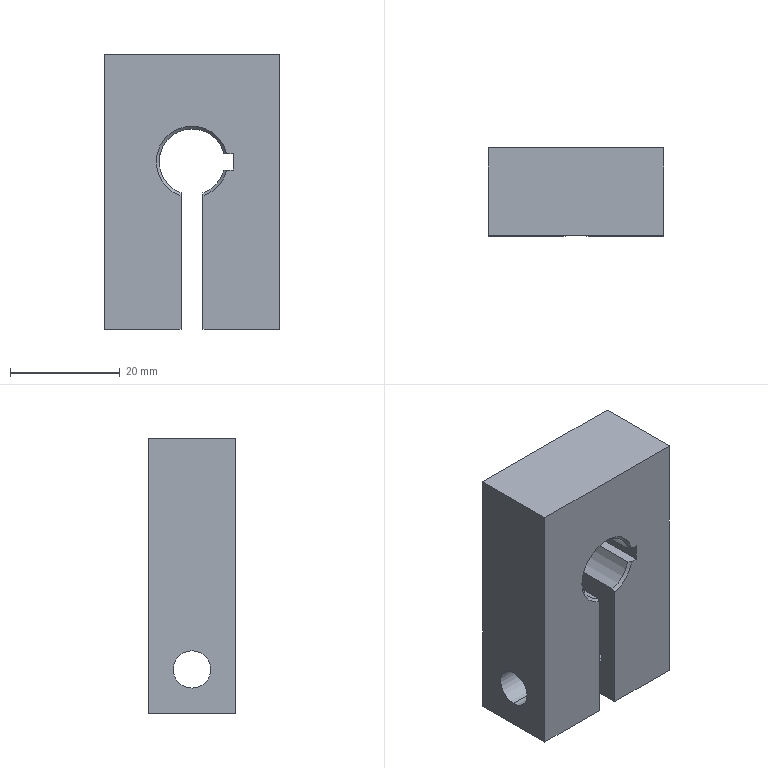Part | SolidWorks | features Chamfer 2, ICE 2, FlatPattern 1, HoleWzd 1, SMBaseFlange 1, SheetMetal 1 | 1 solid | 25 faces | box 32 x 16 x 50 mm | volume 20733 mm3 | plane 14 | cylinder 6 | cone 5 | commonest cylinder face diameters 6.8 x2 9 x2 12 x2
STEP:
#1=CARTESIAN_POINT('',(16.,15.5,-13.5));
#2=VERTEX_POINT('',#1);
#3=CARTESIAN_POINT('',(21.809,15.5,-18.));
#4=VERTEX_POINT('',#3);
#5=CARTESIAN_POINT('',(16.,15.5,-19.5));
#6=DIRECTION('',(0.,1.,0.));
#7=DIRECTION('',(0.,0.,1.));
#8=AXIS2_PLACEMENT_3D('',#5,#6,#7);
#9=CIRCLE('',#8,6.);
#10=EDGE_CURVE('',#2,#4,#9,.T.);
#11=ORIENTED_EDGE('',*,*,#10,.F.);
#12=CARTESIAN_POINT('',(16.,16.,-13.));
#13=VERTEX_POINT('',#12);
#14=CARTESIAN_POINT('',(16.,16.,-13.));
#15=DIRECTION('',(0.,0.7071,0.7071));
#16=VECTOR('',#15,1000.);
#17=LINE('',#14,#16);
#18=EDGE_CURVE('',#2,#13,#17,.T.);
#19=ORIENTED_EDGE('',*,*,#18,.T.);
#20=CARTESIAN_POINT('',(22.246,16.,-17.7));
#21=VERTEX_POINT('',#20);
#22=CARTESIAN_POINT('',(16.,16.,-19.5));
#23=DIRECTION('',(0.,-1.,0.));
#24=DIRECTION('',(0.,0.,1.));
#25=AXIS2_PLACEMENT_3D('',#22,#23,#24);
#26=CIRCLE('',#25,6.5);
#27=EDGE_CURVE('',#21,#13,#26,.T.);
#28=ORIENTED_EDGE('',*,*,#27,.F.);
#29=CARTESIAN_POINT('',(22.016,15.7,-18.));
#30=VERTEX_POINT('',#29);
#31=CARTESIAN_POINT('',(22.246,16.,-17.7));
#32=CARTESIAN_POINT('',(22.17,15.9,-17.8));
#33=CARTESIAN_POINT('',(22.094,15.8,-17.9));
#34=CARTESIAN_POINT('',(22.016,15.7,-18.));
#35=B_SPLINE_CURVE_WITH_KNOTS('',3,(#31,#32,#33,#34),.UNSPECIFIED.,.F.,.F.,(4,4),(0.,0.0004826),.UNSPECIFIED.);
#36=EDGE_CURVE('',#21,#30,#35,.T.);
#37=ORIENTED_EDGE('',*,*,#36,.T.);
#38=CARTESIAN_POINT('',(21.809,15.5,-18.));
#39=CARTESIAN_POINT('',(21.878,15.567,-18.));
#40=CARTESIAN_POINT('',(21.947,15.633,-18.));
#41=CARTESIAN_POINT('',(22.016,15.7,-18.));
#42=B_SPLINE_CURVE_WITH_KNOTS('',3,(#38,#39,#40,#41),.UNSPECIFIED.,.F.,.F.,(4,4),(0.,0.0002874),.UNSPECIFIED.);
#43=EDGE_CURVE('',#4,#30,#42,.T.);
#44=ORIENTED_EDGE('',*,*,#43,.F.);
#45=EDGE_LOOP('',(#11,#19,#28,#37,#44));
#46=FACE_OUTER_BOUND('',#45,.T.);
#47=CARTESIAN_POINT('',(16.,16.,-19.5));
#48=DIRECTION('',(0.,1.,0.));
#49=DIRECTION('',(0.,0.,1.));
#50=AXIS2_PLACEMENT_3D('',#47,#48,#49);
#51=CONICAL_SURFACE('',#50,6.5,0.7854);
#52=ADVANCED_FACE('',(#46),#51,.F.);
#53=CARTESIAN_POINT('',(14.,8.,-45.4));
#54=VERTEX_POINT('',#53);
#55=CARTESIAN_POINT('',(14.,8.,-38.6));
#56=VERTEX_POINT('',#55);
#57=CARTESIAN_POINT('',(14.,8.,-42.));
#58=DIRECTION('',(-1.,0.,0.));
#59=DIRECTION('',(0.,0.,1.));
#60=AXIS2_PLACEMENT_3D('',#57,#58,#59);
#61=CIRCLE('',#60,3.4);
#62=EDGE_CURVE('',#54,#56,#61,.T.);
#63=ORIENTED_EDGE('',*,*,#62,.F.);
#64=CARTESIAN_POINT('',(0.,8.,-45.4));
#65=VERTEX_POINT('',#64);
#66=CARTESIAN_POINT('',(0.,8.,-45.4));
#67=DIRECTION('',(-1.,0.,0.));
#68=VECTOR('',#67,1000.);
#69=LINE('',#66,#68);
#70=EDGE_CURVE('',#54,#65,#69,.T.);
#71=ORIENTED_EDGE('',*,*,#70,.T.);
#72=CARTESIAN_POINT('',(0.,8.,-38.6));
#73=VERTEX_POINT('',#72);
#74=CARTESIAN_POINT('',(0.,8.,-42.));
#75=DIRECTION('',(-1.,0.,0.));
#76=DIRECTION('',(0.,0.,1.));
#77=AXIS2_PLACEMENT_3D('',#74,#75,#76);
#78=CIRCLE('',#77,3.4);
#79=EDGE_CURVE('',#65,#73,#78,.T.);
#80=ORIENTED_EDGE('',*,*,#79,.T.);
#81=CARTESIAN_POINT('',(0.,8.,-38.6));
#82=DIRECTION('',(-1.,0.,0.));
#83=VECTOR('',#82,1000.);
#84=LINE('',#81,#83);
#85=EDGE_CURVE('',#56,#73,#84,.T.);
#86=ORIENTED_EDGE('',*,*,#85,.F.);
#87=EDGE_LOOP('',(#63,#71,#80,#86));
#88=FACE_OUTER_BOUND('',#87,.T.);
#89=CARTESIAN_POINT('',(0.,8.,-42.));
#90=DIRECTION('',(-1.,0.,0.));
#91=DIRECTION('',(0.,0.,1.));
#92=AXIS2_PLACEMENT_3D('',#89,#90,#91);
#93=CYLINDRICAL_SURFACE('',#92,3.4);
#94=ADVANCED_FACE('',(#88),#93,.F.);
#95=CARTESIAN_POINT('',(18.,8.,-46.5));
#96=VERTEX_POINT('',#95);
#97=CARTESIAN_POINT('',(18.,8.,-37.5));
#98=VERTEX_POINT('',#97);
#99=CARTESIAN_POINT('',(18.,8.,-42.));
#100=DIRECTION('',(-1.,0.,0.));
#101=DIRECTION('',(0.,0.,-1.));
#102=AXIS2_PLACEMENT_3D('',#99,#100,#101);
#103=CIRCLE('',#102,4.5);
#104=EDGE_CURVE('',#96,#98,#103,.T.);
#105=ORIENTED_EDGE('',*,*,#104,.T.);
#106=CARTESIAN_POINT('',(32.,8.,-37.5));
#107=VERTEX_POINT('',#106);
#108=CARTESIAN_POINT('',(-0.001,8.,-37.5));
#109=DIRECTION('',(1.,0.,0.));
#110=VECTOR('',#109,1000.);
#111=LINE('',#108,#110);
#112=EDGE_CURVE('',#98,#107,#111,.T.);
#113=ORIENTED_EDGE('',*,*,#112,.T.);
#114=CARTESIAN_POINT('',(32.,8.,-46.5));
#115=VERTEX_POINT('',#114);
#116=CARTESIAN_POINT('',(32.,8.,-42.));
#117=DIRECTION('',(1.,0.,0.));
#118=DIRECTION('',(0.,0.,-1.));
#119=AXIS2_PLACEMENT_3D('',#116,#117,#118);
#120=CIRCLE('',#119,4.5);
#121=EDGE_CURVE('',#107,#115,#120,.T.);
#122=ORIENTED_EDGE('',*,*,#121,.T.);
#123=CARTESIAN_POINT('',(-0.001,8.,-46.5));
#124=DIRECTION('',(1.,0.,0.));
#125=VECTOR('',#124,1000.);
#126=LINE('',#123,#125);
#127=EDGE_CURVE('',#96,#115,#126,.T.);
#128=ORIENTED_EDGE('',*,*,#127,.F.);
#129=EDGE_LOOP('',(#105,#113,#122,#128));
#130=FACE_OUTER_BOUND('',#129,.T.);
#131=CARTESIAN_POINT('',(-0.001,8.,-42.));
#132=DIRECTION('',(1.,0.,0.));
#133=DIRECTION('',(0.,0.,-1.));
#134=AXIS2_PLACEMENT_3D('',#131,#132,#133);
#135=CYLINDRICAL_SURFACE('',#134,4.5);
#136=ADVANCED_FACE('',(#130),#135,.F.);
#137=CARTESIAN_POINT('',(0.,8.,-42.));
#138=DIRECTION('',(-1.,0.,0.));
#139=DIRECTION('',(0.,0.,1.));
#140=AXIS2_PLACEMENT_3D('',#137,#138,#139);
#141=CIRCLE('',#140,3.4);
#142=EDGE_CURVE('',#73,#65,#141,.T.);
#143=ORIENTED_EDGE('',*,*,#142,.F.);
#144=ORIENTED_EDGE('',*,*,#79,.F.);
#145=EDGE_LOOP('',(#143,#144));
#146=FACE_BOUND('',#145,.T.);
#147=CARTESIAN_POINT('',(0.,0.,-50.));
#148=VERTEX_POINT('',#147);
#149=CARTESIAN_POINT('',(0.,0.,0.));
#150=VERTEX_POINT('',#149);
#151=CARTESIAN_POINT('',(0.,0.,0.));
#152=DIRECTION('',(0.,0.,1.));
#153=VECTOR('',#152,1000.);
#154=LINE('',#151,#153);
#155=EDGE_CURVE('',#148,#150,#154,.T.);
#156=ORIENTED_EDGE('',*,*,#155,.T.);
#157=CARTESIAN_POINT('',(0.,16.,0.));
#158=VERTEX_POINT('',#157);
#159=CARTESIAN_POINT('',(0.,16.,0.));
#160=DIRECTION('',(0.,-1.,0.));
#161=VECTOR('',#160,1000.);
#162=LINE('',#159,#161);
#163=EDGE_CURVE('',#158,#150,#162,.T.);
#164=ORIENTED_EDGE('',*,*,#163,.F.);
#165=CARTESIAN_POINT('',(0.,16.,-50.));
#166=VERTEX_POINT('',#165);
#167=CARTESIAN_POINT('',(0.,16.,0.));
#168=DIRECTION('',(0.,0.,1.));
#169=VECTOR('',#168,1000.);
#170=LINE('',#167,#169);
#171=EDGE_CURVE('',#166,#158,#170,.T.);
#172=ORIENTED_EDGE('',*,*,#171,.F.);
#173=CARTESIAN_POINT('',(0.,16.,-50.));
#174=DIRECTION('',(0.,-1.,0.));
#175=VECTOR('',#174,1000.);
#176=LINE('',#173,#175);
#177=EDGE_CURVE('',#166,#148,#176,.T.);
#178=ORIENTED_EDGE('',*,*,#177,.T.);
#179=EDGE_LOOP('',(#156,#164,#172,#178));
#180=FACE_OUTER_BOUND('',#179,.T.);
#181=CARTESIAN_POINT('',(0.,16.,0.));
#182=DIRECTION('',(1.,0.,0.));
#183=DIRECTION('',(0.,0.,-1.));
#184=AXIS2_PLACEMENT_3D('',#181,#182,#183);
#185=PLANE('',#184);
#186=ADVANCED_FACE('',(#146,#180),#185,.F.);
#187=CARTESIAN_POINT('',(32.,0.,0.));
#188=VERTEX_POINT('',#187);
#189=CARTESIAN_POINT('',(0.,0.,0.));
#190=DIRECTION('',(1.,0.,0.));
#191=VECTOR('',#190,1000.);
#192=LINE('',#189,#191);
#193=EDGE_CURVE('',#150,#188,#192,.T.);
#194=ORIENTED_EDGE('',*,*,#193,.T.);
#195=CARTESIAN_POINT('',(32.,16.,0.));
#196=VERTEX_POINT('',#195);
#197=CARTESIAN_POINT('',(32.,16.,0.));
#198=DIRECTION('',(0.,-1.,0.));
#199=VECTOR('',#198,1000.);
#200=LINE('',#197,#199);
#201=EDGE_CURVE('',#196,#188,#200,.T.);
#202=ORIENTED_EDGE('',*,*,#201,.F.);
#203=CARTESIAN_POINT('',(0.,16.,0.));
#204=DIRECTION('',(1.,0.,0.));
#205=VECTOR('',#204,1000.);
#206=LINE('',#203,#205);
#207=EDGE_CURVE('',#158,#196,#206,.T.);
#208=ORIENTED_EDGE('',*,*,#207,.F.);
#209=ORIENTED_EDGE('',*,*,#163,.T.);
#210=EDGE_LOOP('',(#194,#202,#208,#209));
#211=FACE_OUTER_BOUND('',#210,.T.);
#212=CARTESIAN_POINT('',(0.,16.,0.));
#213=DIRECTION('',(0.,0.,-1.));
#214=DIRECTION('',(-1.,0.,0.));
#215=AXIS2_PLACEMENT_3D('',#212,#213,#214);
#216=PLANE('',#215);
#217=ADVANCED_FACE('',(#211),#216,.F.);
#218=CARTESIAN_POINT('',(32.,8.,-42.));
#219=DIRECTION('',(1.,0.,0.));
#220=DIRECTION('',(0.,0.,-1.));
#221=AXIS2_PLACEMENT_3D('',#218,#219,#220);
#222=CIRCLE('',#221,4.5);
#223=EDGE_CURVE('',#115,#107,#222,.T.);
#224=ORIENTED_EDGE('',*,*,#223,.F.);
#225=ORIENTED_EDGE('',*,*,#121,.F.);
#226=EDGE_LOOP('',(#224,#225));
#227=FACE_BOUND('',#226,.T.);
#228=CARTESIAN_POINT('',(32.,0.,-50.));
#229=VERTEX_POINT('',#228);
#230=CARTESIAN_POINT('',(32.,0.,0.));
#231=DIRECTION('',(0.,0.,-1.));
#232=VECTOR('',#231,1000.);
#233=LINE('',#230,#232);
#234=EDGE_CURVE('',#188,#229,#233,.T.);
#235=ORIENTED_EDGE('',*,*,#234,.T.);
#236=CARTESIAN_POINT('',(32.,16.,-50.));
#237=VERTEX_POINT('',#236);
#238=CARTESIAN_POINT('',(32.,16.,-50.));
#239=DIRECTION('',(0.,-1.,0.));
#240=VECTOR('',#239,1000.);
#241=LINE('',#238,#240);
#242=EDGE_CURVE('',#237,#229,#241,.T.);
#243=ORIENTED_EDGE('',*,*,#242,.F.);
#244=CARTESIAN_POINT('',(32.,16.,0.));
#245=DIRECTION('',(0.,0.,-1.));
#246=VECTOR('',#245,1000.);
#247=LINE('',#244,#246);
#248=EDGE_CURVE('',#196,#237,#247,.T.);
#249=ORIENTED_EDGE('',*,*,#248,.F.);
#250=ORIENTED_EDGE('',*,*,#201,.T.);
#251=EDGE_LOOP('',(#235,#243,#249,#250));
#252=FACE_OUTER_BOUND('',#251,.T.);
#253=CARTESIAN_POINT('',(32.,16.,0.));
#254=DIRECTION('',(-1.,0.,0.));
#255=DIRECTION('',(0.,0.,1.));
#256=AXIS2_PLACEMENT_3D('',#253,#254,#255);
#257=PLANE('',#256);
#258=ADVANCED_FACE('',(#227,#252),#257,.F.);
#259=CARTESIAN_POINT('',(18.,0.,-50.));
#260=VERTEX_POINT('',#259);
#261=CARTESIAN_POINT('',(18.,0.,-50.));
#262=DIRECTION('',(-1.,0.,0.));
#263=VECTOR('',#262,1000.);
#264=LINE('',#261,#263);
#265=EDGE_CURVE('',#229,#260,#264,.T.);
#266=ORIENTED_EDGE('',*,*,#265,.T.);
#267=CARTESIAN_POINT('',(18.,16.,-50.));
#268=VERTEX_POINT('',#267);
#269=CARTESIAN_POINT('',(18.,16.,-50.));
#270=DIRECTION('',(0.,-1.,0.));
#271=VECTOR('',#270,1000.);
#272=LINE('',#269,#271);
#273=EDGE_CURVE('',#268,#260,#272,.T.);
#274=ORIENTED_EDGE('',*,*,#273,.F.);
#275=CARTESIAN_POINT('',(18.,16.,-50.));
#276=DIRECTION('',(-1.,0.,0.));
#277=VECTOR('',#276,1000.);
#278=LINE('',#275,#277);
#279=EDGE_CURVE('',#237,#268,#278,.T.);
#280=ORIENTED_EDGE('',*,*,#279,.F.);
#281=ORIENTED_EDGE('',*,*,#242,.T.);
#282=EDGE_LOOP('',(#266,#274,#280,#281));
#283=FACE_OUTER_BOUND('',#282,.T.);
#284=CARTESIAN_POINT('',(18.,16.,-50.));
#285=DIRECTION('',(0.,0.,1.));
#286=DIRECTION('',(1.,0.,0.));
#287=AXIS2_PLACEMENT_3D('',#284,#285,#286);
#288=PLANE('',#287);
#289=ADVANCED_FACE('',(#283),#288,.F.);
#290=ORIENTED_EDGE('',*,*,#104,.F.);
#291=CARTESIAN_POINT('',(18.,8.,-42.));
#292=DIRECTION('',(-1.,0.,0.));
#293=DIRECTION('',(0.,0.,-1.));
#294=AXIS2_PLACEMENT_3D('',#291,#292,#293);
#295=CIRCLE('',#294,4.5);
#296=EDGE_CURVE('',#98,#96,#295,.T.);
#297=ORIENTED_EDGE('',*,*,#296,.F.);
#298=EDGE_LOOP('',(#290,#297));
#299=FACE_BOUND('',#298,.T.);
#300=CARTESIAN_POINT('',(18.,0.,-25.685));
#301=VERTEX_POINT('',#300);
#302=CARTESIAN_POINT('',(18.,0.,-50.));
#303=DIRECTION('',(0.,0.,1.));
#304=VECTOR('',#303,1000.);
#305=LINE('',#302,#304);
#306=EDGE_CURVE('',#260,#301,#305,.T.);
#307=ORIENTED_EDGE('',*,*,#306,.T.);
#308=CARTESIAN_POINT('',(18.,0.5,-25.157));
#309=VERTEX_POINT('',#308);
#310=CARTESIAN_POINT('',(18.,0.,-25.685));
#311=CARTESIAN_POINT('',(18.,0.1671,-25.509));
#312=CARTESIAN_POINT('',(18.,0.3338,-25.333));
#313=CARTESIAN_POINT('',(18.,0.5,-25.157));
#314=B_SPLINE_CURVE_WITH_KNOTS('',3,(#310,#311,#312,#313),.UNSPECIFIED.,.F.,.F.,(4,4),(0.,0.000727),.UNSPECIFIED.);
#315=EDGE_CURVE('',#301,#309,#314,.T.);
#316=ORIENTED_EDGE('',*,*,#315,.T.);
#317=CARTESIAN_POINT('',(18.,15.5,-25.157));
#318=VERTEX_POINT('',#317);
#319=CARTESIAN_POINT('',(18.,16.,-25.157));
#320=DIRECTION('',(0.,-1.,0.));
#321=VECTOR('',#320,1000.);
#322=LINE('',#319,#321);
#323=EDGE_CURVE('',#318,#309,#322,.T.);
#324=ORIENTED_EDGE('',*,*,#323,.F.);
#325=CARTESIAN_POINT('',(18.,16.,-25.685));
#326=VERTEX_POINT('',#325);
#327=CARTESIAN_POINT('',(18.,15.5,-25.157));
#328=CARTESIAN_POINT('',(18.,15.666,-25.333));
#329=CARTESIAN_POINT('',(18.,15.833,-25.509));
#330=CARTESIAN_POINT('',(18.,16.,-25.685));
#331=B_SPLINE_CURVE_WITH_KNOTS('',3,(#327,#328,#329,#330),.UNSPECIFIED.,.F.,.F.,(4,4),(0.,0.000727),.UNSPECIFIED.);
#332=EDGE_CURVE('',#318,#326,#331,.T.);
#333=ORIENTED_EDGE('',*,*,#332,.T.);
#334=CARTESIAN_POINT('',(18.,16.,-50.));
#335=DIRECTION('',(0.,0.,1.));
#336=VECTOR('',#335,1000.);
#337=LINE('',#334,#336);
#338=EDGE_CURVE('',#268,#326,#337,.T.);
#339=ORIENTED_EDGE('',*,*,#338,.F.);
#340=ORIENTED_EDGE('',*,*,#273,.T.);
#341=EDGE_LOOP('',(#307,#316,#324,#333,#339,#340));
#342=FACE_OUTER_BOUND('',#341,.T.);
#343=CARTESIAN_POINT('',(18.,16.,-50.));
#344=DIRECTION('',(1.,0.,0.));
#345=DIRECTION('',(0.,0.,-1.));
#346=AXIS2_PLACEMENT_3D('',#343,#344,#345);
#347=PLANE('',#346);
#348=ADVANCED_FACE('',(#299,#342),#347,.F.);
#349=ORIENTED_EDGE('',*,*,#323,.T.);
#350=CARTESIAN_POINT('',(21.809,0.5,-21.));
#351=VERTEX_POINT('',#350);
#352=CARTESIAN_POINT('',(16.,0.5,-19.5));
#353=DIRECTION('',(0.,-1.,0.));
#354=DIRECTION('',(0.,0.,1.));
#355=AXIS2_PLACEMENT_3D('',#352,#353,#354);
#356=CIRCLE('',#355,6.);
#357=EDGE_CURVE('',#309,#351,#356,.T.);
#358=ORIENTED_EDGE('',*,*,#357,.T.);
#359=CARTESIAN_POINT('',(21.809,15.5,-21.));
#360=VERTEX_POINT('',#359);
#361=CARTESIAN_POINT('',(21.809,16.,-21.));
#362=DIRECTION('',(0.,-1.,0.));
#363=VECTOR('',#362,1000.);
#364=LINE('',#361,#363);
#365=EDGE_CURVE('',#360,#351,#364,.T.);
#366=ORIENTED_EDGE('',*,*,#365,.F.);
#367=CARTESIAN_POINT('',(16.,15.5,-19.5));
#368=DIRECTION('',(0.,1.,0.));
#369=DIRECTION('',(0.,0.,1.));
#370=AXIS2_PLACEMENT_3D('',#367,#368,#369);
#371=CIRCLE('',#370,6.);
#372=EDGE_CURVE('',#360,#318,#371,.T.);
#373=ORIENTED_EDGE('',*,*,#372,.T.);
#374=EDGE_LOOP('',(#349,#358,#366,#373));
#375=FACE_OUTER_BOUND('',#374,.T.);
#376=CARTESIAN_POINT('',(16.,16.,-19.5));
#377=DIRECTION('',(0.,-1.,0.));
#378=DIRECTION('',(0.,0.,-1.));
#379=AXIS2_PLACEMENT_3D('',#376,#377,#378);
#380=CYLINDRICAL_SURFACE('',#379,6.);
#381=ADVANCED_FACE('',(#375),#380,.F.);
#382=CARTESIAN_POINT('',(23.5,15.7,-21.));
#383=VERTEX_POINT('',#382);
#384=CARTESIAN_POINT('',(23.5,0.,-21.));
#385=VERTEX_POINT('',#384);
#386=CARTESIAN_POINT('',(23.5,16.,-21.));
#387=DIRECTION('',(0.,-1.,0.));
#388=VECTOR('',#387,1000.);
#389=LINE('',#386,#388);
#390=EDGE_CURVE('',#383,#385,#389,.T.);
#391=ORIENTED_EDGE('',*,*,#390,.F.);
#392=CARTESIAN_POINT('',(22.016,15.7,-21.));
#393=VERTEX_POINT('',#392);
#394=CARTESIAN_POINT('',(22.325,15.7,-21.));
#395=DIRECTION('',(-1.,0.,0.));
#396=VECTOR('',#395,1000.);
#397=LINE('',#394,#396);
#398=EDGE_CURVE('',#383,#393,#397,.T.);
#399=ORIENTED_EDGE('',*,*,#398,.T.);
#400=CARTESIAN_POINT('',(22.016,15.7,-21.));
#401=CARTESIAN_POINT('',(21.947,15.633,-21.));
#402=CARTESIAN_POINT('',(21.878,15.567,-21.));
#403=CARTESIAN_POINT('',(21.809,15.5,-21.));
#404=B_SPLINE_CURVE_WITH_KNOTS('',3,(#400,#401,#402,#403),.UNSPECIFIED.,.F.,.F.,(4,4),(0.0004305,0.0007178),.UNSPECIFIED.);
#405=EDGE_CURVE('',#393,#360,#404,.T.);
#406=ORIENTED_EDGE('',*,*,#405,.T.);
#407=ORIENTED_EDGE('',*,*,#365,.T.);
#408=CARTESIAN_POINT('',(22.325,0.,-21.));
#409=VERTEX_POINT('',#408);
#410=CARTESIAN_POINT('',(21.809,0.5,-21.));
#411=CARTESIAN_POINT('',(21.981,0.3336,-21.));
#412=CARTESIAN_POINT('',(22.153,0.1669,-21.));
#413=CARTESIAN_POINT('',(22.325,0.,-21.));
#414=B_SPLINE_CURVE_WITH_KNOTS('',3,(#410,#411,#412,#413),.UNSPECIFIED.,.F.,.F.,(4,4),(0.,0.0007178),.UNSPECIFIED.);
#415=EDGE_CURVE('',#351,#409,#414,.T.);
#416=ORIENTED_EDGE('',*,*,#415,.T.);
#417=CARTESIAN_POINT('',(21.809,0.,-21.));
#418=DIRECTION('',(1.,0.,0.));
#419=VECTOR('',#418,1000.);
#420=LINE('',#417,#419);
#421=EDGE_CURVE('',#409,#385,#420,.T.);
#422=ORIENTED_EDGE('',*,*,#421,.T.);
#423=EDGE_LOOP('',(#391,#399,#406,#407,#416,#422));
#424=FACE_OUTER_BOUND('',#423,.T.);
#425=CARTESIAN_POINT('',(21.809,16.,-21.));
#426=DIRECTION('',(0.,0.,-1.));
#427=DIRECTION('',(-1.,0.,0.));
#428=AXIS2_PLACEMENT_3D('',#425,#426,#427);
#429=PLANE('',#428);
#430=ADVANCED_FACE('',(#424),#429,.F.);
#431=CARTESIAN_POINT('',(23.5,0.,-18.));
#432=VERTEX_POINT('',#431);
#433=CARTESIAN_POINT('',(23.5,0.,-21.));
#434=DIRECTION('',(0.,0.,1.));
#435=VECTOR('',#434,1000.);
#436=LINE('',#433,#435);
#437=EDGE_CURVE('',#385,#432,#436,.T.);
#438=ORIENTED_EDGE('',*,*,#437,.T.);
#439=CARTESIAN_POINT('',(23.5,15.7,-18.));
#440=VERTEX_POINT('',#439);
#441=CARTESIAN_POINT('',(23.5,16.,-18.));
#442=DIRECTION('',(0.,-1.,0.));
#443=VECTOR('',#442,1000.);
#444=LINE('',#441,#443);
#445=EDGE_CURVE('',#440,#432,#444,.T.);
#446=ORIENTED_EDGE('',*,*,#445,.F.);
#447=CARTESIAN_POINT('',(23.5,16.,-17.7));
#448=VERTEX_POINT('',#447);
#449=CARTESIAN_POINT('',(23.5,14.35,-19.35));
#450=DIRECTION('',(0.,0.7071,0.7071));
#451=VECTOR('',#450,1000.);
#452=LINE('',#449,#451);
#453=EDGE_CURVE('',#440,#448,#452,.T.);
#454=ORIENTED_EDGE('',*,*,#453,.T.);
#455=CARTESIAN_POINT('',(23.5,16.,-21.3));
#456=VERTEX_POINT('',#455);
#457=CARTESIAN_POINT('',(23.5,16.,-21.));
#458=DIRECTION('',(0.,0.,1.));
#459=VECTOR('',#458,1000.);
#460=LINE('',#457,#459);
#461=EDGE_CURVE('',#456,#448,#460,.T.);
#462=ORIENTED_EDGE('',*,*,#461,.F.);
#463=CARTESIAN_POINT('',(23.5,15.85,-21.15));
#464=DIRECTION('',(0.,-0.7071,0.7071));
#465=VECTOR('',#464,1000.);
#466=LINE('',#463,#465);
#467=EDGE_CURVE('',#456,#383,#466,.T.);
#468=ORIENTED_EDGE('',*,*,#467,.T.);
#469=ORIENTED_EDGE('',*,*,#390,.T.);
#470=EDGE_LOOP('',(#438,#446,#454,#462,#468,#469));
#471=FACE_OUTER_BOUND('',#470,.T.);
#472=CARTESIAN_POINT('',(23.5,16.,-21.));
#473=DIRECTION('',(1.,0.,0.));
#474=DIRECTION('',(0.,0.,-1.));
#475=AXIS2_PLACEMENT_3D('',#472,#473,#474);
#476=PLANE('',#475);
#477=ADVANCED_FACE('',(#471),#476,.F.);
#478=ORIENTED_EDGE('',*,*,#43,.T.);
#479=CARTESIAN_POINT('',(23.5,15.7,-18.));
#480=DIRECTION('',(1.,0.,0.));
#481=VECTOR('',#480,1000.);
#482=LINE('',#479,#481);
#483=EDGE_CURVE('',#30,#440,#482,.T.);
#484=ORIENTED_EDGE('',*,*,#483,.T.);
#485=ORIENTED_EDGE('',*,*,#445,.T.);
#486=CARTESIAN_POINT('',(22.325,0.,-18.));
#487=VERTEX_POINT('',#486);
#488=CARTESIAN_POINT('',(21.809,0.,-18.));
#489=DIRECTION('',(-1.,0.,0.));
#490=VECTOR('',#489,1000.);
#491=LINE('',#488,#490);
#492=EDGE_CURVE('',#432,#487,#491,.T.);
#493=ORIENTED_EDGE('',*,*,#492,.T.);
#494=CARTESIAN_POINT('',(21.809,0.5,-18.));
#495=VERTEX_POINT('',#494);
#496=CARTESIAN_POINT('',(22.325,0.,-18.));
#497=CARTESIAN_POINT('',(22.153,0.1669,-18.));
#498=CARTESIAN_POINT('',(21.981,0.3336,-18.));
#499=CARTESIAN_POINT('',(21.809,0.5,-18.));
#500=B_SPLINE_CURVE_WITH_KNOTS('',3,(#496,#497,#498,#499),.UNSPECIFIED.,.F.,.F.,(4,4),(0.,0.0007178),.UNSPECIFIED.);
#501=EDGE_CURVE('',#487,#495,#500,.T.);
#502=ORIENTED_EDGE('',*,*,#501,.T.);
#503=CARTESIAN_POINT('',(21.809,16.,-18.));
#504=DIRECTION('',(0.,-1.,0.));
#505=VECTOR('',#504,1000.);
#506=LINE('',#503,#505);
#507=EDGE_CURVE('',#4,#495,#506,.T.);
#508=ORIENTED_EDGE('',*,*,#507,.F.);
#509=EDGE_LOOP('',(#478,#484,#485,#493,#502,#508));
#510=FACE_OUTER_BOUND('',#509,.T.);
#511=CARTESIAN_POINT('',(21.809,16.,-18.));
#512=DIRECTION('',(0.,0.,1.));
#513=DIRECTION('',(1.,0.,0.));
#514=AXIS2_PLACEMENT_3D('',#511,#512,#513);
#515=PLANE('',#514);
#516=ADVANCED_FACE('',(#510),#515,.F.);
#517=ORIENTED_EDGE('',*,*,#507,.T.);
#518=CARTESIAN_POINT('',(14.,0.5,-25.157));
#519=VERTEX_POINT('',#518);
#520=CARTESIAN_POINT('',(16.,0.5,-19.5));
#521=DIRECTION('',(0.,-1.,0.));
#522=DIRECTION('',(0.,0.,1.));
#523=AXIS2_PLACEMENT_3D('',#520,#521,#522);
#524=CIRCLE('',#523,6.);
#525=EDGE_CURVE('',#495,#519,#524,.T.);
#526=ORIENTED_EDGE('',*,*,#525,.T.);
#527=CARTESIAN_POINT('',(14.,15.5,-25.157));
#528=VERTEX_POINT('',#527);
#529=CARTESIAN_POINT('',(14.,16.,-25.157));
#530=DIRECTION('',(0.,-1.,0.));
#531=VECTOR('',#530,1000.);
#532=LINE('',#529,#531);
#533=EDGE_CURVE('',#528,#519,#532,.T.);
#534=ORIENTED_EDGE('',*,*,#533,.F.);
#535=CARTESIAN_POINT('',(16.,15.5,-19.5));
#536=DIRECTION('',(0.,1.,0.));
#537=DIRECTION('',(0.,0.,1.));
#538=AXIS2_PLACEMENT_3D('',#535,#536,#537);
#539=CIRCLE('',#538,6.);
#540=EDGE_CURVE('',#528,#2,#539,.T.);
#541=ORIENTED_EDGE('',*,*,#540,.T.);
#542=ORIENTED_EDGE('',*,*,#10,.T.);
#543=EDGE_LOOP('',(#517,#526,#534,#541,#542));
#544=FACE_OUTER_BOUND('',#543,.T.);
#545=CARTESIAN_POINT('',(16.,16.,-19.5));
#546=DIRECTION('',(0.,-1.,0.));
#547=DIRECTION('',(0.,0.,-1.));
#548=AXIS2_PLACEMENT_3D('',#545,#546,#547);
#549=CYLINDRICAL_SURFACE('',#548,6.);
#550=ADVANCED_FACE('',(#544),#549,.F.);
#551=CARTESIAN_POINT('',(14.,8.,-42.));
#552=DIRECTION('',(-1.,0.,0.));
#553=DIRECTION('',(0.,0.,1.));
#554=AXIS2_PLACEMENT_3D('',#551,#552,#553);
#555=CIRCLE('',#554,3.4);
#556=EDGE_CURVE('',#56,#54,#555,.T.);
#557=ORIENTED_EDGE('',*,*,#556,.T.);
#558=ORIENTED_EDGE('',*,*,#62,.T.);
#559=EDGE_LOOP('',(#557,#558));
#560=FACE_BOUND('',#559,.T.);
#561=ORIENTED_EDGE('',*,*,#533,.T.);
#562=CARTESIAN_POINT('',(14.,0.,-25.685));
#563=VERTEX_POINT('',#562);
#564=CARTESIAN_POINT('',(14.,0.5,-25.157));
#565=CARTESIAN_POINT('',(14.,0.3338,-25.333));
#566=CARTESIAN_POINT('',(14.,0.1671,-25.509));
#567=CARTESIAN_POINT('',(14.,0.,-25.685));
#568=B_SPLINE_CURVE_WITH_KNOTS('',3,(#564,#565,#566,#567),.UNSPECIFIED.,.F.,.F.,(4,4),(0.,0.000727),.UNSPECIFIED.);
#569=EDGE_CURVE('',#519,#563,#568,.T.);
#570=ORIENTED_EDGE('',*,*,#569,.T.);
#571=CARTESIAN_POINT('',(14.,0.,-50.));
#572=VERTEX_POINT('',#571);
#573=CARTESIAN_POINT('',(14.,0.,-50.));
#574=DIRECTION('',(0.,0.,-1.));
#575=VECTOR('',#574,1000.);
#576=LINE('',#573,#575);
#577=EDGE_CURVE('',#563,#572,#576,.T.);
#578=ORIENTED_EDGE('',*,*,#577,.T.);
#579=CARTESIAN_POINT('',(14.,16.,-50.));
#580=VERTEX_POINT('',#579);
#581=CARTESIAN_POINT('',(14.,16.,-50.));
#582=DIRECTION('',(0.,-1.,0.));
#583=VECTOR('',#582,1000.);
#584=LINE('',#581,#583);
#585=EDGE_CURVE('',#580,#572,#584,.T.);
#586=ORIENTED_EDGE('',*,*,#585,.F.);
#587=CARTESIAN_POINT('',(14.,16.,-25.685));
#588=VERTEX_POINT('',#587);
#589=CARTESIAN_POINT('',(14.,16.,-50.));
#590=DIRECTION('',(0.,0.,-1.));
#591=VECTOR('',#590,1000.);
#592=LINE('',#589,#591);
#593=EDGE_CURVE('',#588,#580,#592,.T.);
#594=ORIENTED_EDGE('',*,*,#593,.F.);
#595=CARTESIAN_POINT('',(14.,16.,-25.685));
#596=CARTESIAN_POINT('',(14.,15.833,-25.509));
#597=CARTESIAN_POINT('',(14.,15.666,-25.333));
#598=CARTESIAN_POINT('',(14.,15.5,-25.157));
#599=B_SPLINE_CURVE_WITH_KNOTS('',3,(#595,#596,#597,#598),.UNSPECIFIED.,.F.,.F.,(4,4),(0.,0.000727),.UNSPECIFIED.);
#600=EDGE_CURVE('',#588,#528,#599,.T.);
#601=ORIENTED_EDGE('',*,*,#600,.T.);
#602=EDGE_LOOP('',(#561,#570,#578,#586,#594,#601));
#603=FACE_OUTER_BOUND('',#602,.T.);
#604=CARTESIAN_POINT('',(14.,16.,-50.));
#605=DIRECTION('',(-1.,0.,0.));
#606=DIRECTION('',(0.,0.,1.));
#607=AXIS2_PLACEMENT_3D('',#604,#605,#606);
#608=PLANE('',#607);
#609=ADVANCED_FACE('',(#560,#603),#608,.F.);
#610=CARTESIAN_POINT('',(0.,0.,-50.));
#611=DIRECTION('',(-1.,0.,0.));
#612=VECTOR('',#611,1000.);
#613=LINE('',#610,#612);
#614=EDGE_CURVE('',#572,#148,#613,.T.);
#615=ORIENTED_EDGE('',*,*,#614,.T.);
#616=ORIENTED_EDGE('',*,*,#177,.F.);
#617=CARTESIAN_POINT('',(0.,16.,-50.));
#618=DIRECTION('',(-1.,0.,0.));
#619=VECTOR('',#618,1000.);
#620=LINE('',#617,#619);
#621=EDGE_CURVE('',#580,#166,#620,.T.);
#622=ORIENTED_EDGE('',*,*,#621,.F.);
#623=ORIENTED_EDGE('',*,*,#585,.T.);
#624=EDGE_LOOP('',(#615,#616,#622,#623));
#625=FACE_OUTER_BOUND('',#624,.T.);
#626=CARTESIAN_POINT('',(0.,16.,-50.));
#627=DIRECTION('',(0.,0.,1.));
#628=DIRECTION('',(1.,0.,0.));
#629=AXIS2_PLACEMENT_3D('',#626,#627,#628);
#630=PLANE('',#629);
#631=ADVANCED_FACE('',(#625),#630,.F.);
#632=ORIENTED_EDGE('',*,*,#461,.T.);
#633=CARTESIAN_POINT('',(22.325,16.,-17.7));
#634=DIRECTION('',(-1.,0.,0.));
#635=VECTOR('',#634,1000.);
#636=LINE('',#633,#635);
#637=EDGE_CURVE('',#448,#21,#636,.T.);
#638=ORIENTED_EDGE('',*,*,#637,.T.);
#639=ORIENTED_EDGE('',*,*,#27,.T.);
#640=CARTESIAN_POINT('',(16.,16.,-19.5));
#641=DIRECTION('',(0.,-1.,0.));
#642=DIRECTION('',(0.,0.,1.));
#643=AXIS2_PLACEMENT_3D('',#640,#641,#642);
#644=CIRCLE('',#643,6.5);
#645=EDGE_CURVE('',#13,#588,#644,.T.);
#646=ORIENTED_EDGE('',*,*,#645,.T.);
#647=ORIENTED_EDGE('',*,*,#593,.T.);
#648=ORIENTED_EDGE('',*,*,#621,.T.);
#649=ORIENTED_EDGE('',*,*,#171,.T.);
#650=ORIENTED_EDGE('',*,*,#207,.T.);
#651=ORIENTED_EDGE('',*,*,#248,.T.);
#652=ORIENTED_EDGE('',*,*,#279,.T.);
#653=ORIENTED_EDGE('',*,*,#338,.T.);
#654=CARTESIAN_POINT('',(22.246,16.,-21.3));
#655=VERTEX_POINT('',#654);
#656=CARTESIAN_POINT('',(16.,16.,-19.5));
#657=DIRECTION('',(0.,-1.,0.));
#658=DIRECTION('',(0.,0.,1.));
#659=AXIS2_PLACEMENT_3D('',#656,#657,#658);
#660=CIRCLE('',#659,6.5);
#661=EDGE_CURVE('',#326,#655,#660,.T.);
#662=ORIENTED_EDGE('',*,*,#661,.T.);
#663=CARTESIAN_POINT('',(23.5,16.,-21.3));
#664=DIRECTION('',(1.,0.,0.));
#665=VECTOR('',#664,1000.);
#666=LINE('',#663,#665);
#667=EDGE_CURVE('',#655,#456,#666,.T.);
#668=ORIENTED_EDGE('',*,*,#667,.T.);
#669=EDGE_LOOP('',(#632,#638,#639,#646,#647,#648,#649,#650,#651,#652,#653,#662,#668));
#670=FACE_OUTER_BOUND('',#669,.T.);
#671=CARTESIAN_POINT('',(16.,16.,-19.5));
#672=DIRECTION('',(0.,1.,0.));
#673=DIRECTION('',(0.,0.,1.));
#674=AXIS2_PLACEMENT_3D('',#671,#672,#673);
#675=PLANE('',#674);
#676=ADVANCED_FACE('',(#670),#675,.T.);
#677=ORIENTED_EDGE('',*,*,#421,.F.);
#678=CARTESIAN_POINT('',(16.,0.,-19.5));
#679=DIRECTION('',(0.,1.,0.));
#680=DIRECTION('',(0.,0.,1.));
#681=AXIS2_PLACEMENT_3D('',#678,#679,#680);
#682=CIRCLE('',#681,6.5);
#683=EDGE_CURVE('',#409,#301,#682,.T.);
#684=ORIENTED_EDGE('',*,*,#683,.T.);
#685=ORIENTED_EDGE('',*,*,#306,.F.);
#686=ORIENTED_EDGE('',*,*,#265,.F.);
#687=ORIENTED_EDGE('',*,*,#234,.F.);
#688=ORIENTED_EDGE('',*,*,#193,.F.);
#689=ORIENTED_EDGE('',*,*,#155,.F.);
#690=ORIENTED_EDGE('',*,*,#614,.F.);
#691=ORIENTED_EDGE('',*,*,#577,.F.);
#692=CARTESIAN_POINT('',(16.,0.,-19.5));
#693=DIRECTION('',(0.,1.,0.));
#694=DIRECTION('',(0.,0.,1.));
#695=AXIS2_PLACEMENT_3D('',#692,#693,#694);
#696=CIRCLE('',#695,6.5);
#697=EDGE_CURVE('',#563,#487,#696,.T.);
#698=ORIENTED_EDGE('',*,*,#697,.T.);
#699=ORIENTED_EDGE('',*,*,#492,.F.);
#700=ORIENTED_EDGE('',*,*,#437,.F.);
#701=EDGE_LOOP('',(#677,#684,#685,#686,#687,#688,#689,#690,#691,#698,#699,#700));
#702=FACE_OUTER_BOUND('',#701,.T.);
#703=CARTESIAN_POINT('',(16.,0.,-19.5));
#704=DIRECTION('',(0.,1.,0.));
#705=DIRECTION('',(0.,0.,1.));
#706=AXIS2_PLACEMENT_3D('',#703,#704,#705);
#707=PLANE('',#706);
#708=ADVANCED_FACE('',(#702),#707,.F.);
#709=ORIENTED_EDGE('',*,*,#112,.F.);
#710=ORIENTED_EDGE('',*,*,#296,.T.);
#711=ORIENTED_EDGE('',*,*,#127,.T.);
#712=ORIENTED_EDGE('',*,*,#223,.T.);
#713=EDGE_LOOP('',(#709,#710,#711,#712));
#714=FACE_OUTER_BOUND('',#713,.T.);
#715=CARTESIAN_POINT('',(-0.001,8.,-42.));
#716=DIRECTION('',(1.,0.,0.));
#717=DIRECTION('',(0.,0.,-1.));
#718=AXIS2_PLACEMENT_3D('',#715,#716,#717);
#719=CYLINDRICAL_SURFACE('',#718,4.5);
#720=ADVANCED_FACE('',(#714),#719,.F.);
#721=ORIENTED_EDGE('',*,*,#70,.F.);
#722=ORIENTED_EDGE('',*,*,#556,.F.);
#723=ORIENTED_EDGE('',*,*,#85,.T.);
#724=ORIENTED_EDGE('',*,*,#142,.T.);
#725=EDGE_LOOP('',(#721,#722,#723,#724));
#726=FACE_OUTER_BOUND('',#725,.T.);
#727=CARTESIAN_POINT('',(0.,8.,-42.));
#728=DIRECTION('',(-1.,0.,0.));
#729=DIRECTION('',(0.,0.,1.));
#730=AXIS2_PLACEMENT_3D('',#727,#728,#729);
#731=CYLINDRICAL_SURFACE('',#730,3.4);
#732=ADVANCED_FACE('',(#726),#731,.F.);
#733=ORIENTED_EDGE('',*,*,#315,.F.);
#734=ORIENTED_EDGE('',*,*,#683,.F.);
#735=ORIENTED_EDGE('',*,*,#415,.F.);
#736=ORIENTED_EDGE('',*,*,#357,.F.);
#737=EDGE_LOOP('',(#733,#734,#735,#736));
#738=FACE_OUTER_BOUND('',#737,.T.);
#739=CARTESIAN_POINT('',(16.,0.5,-19.5));
#740=DIRECTION('',(0.,-1.,0.));
#741=DIRECTION('',(0.,0.,-1.));
#742=AXIS2_PLACEMENT_3D('',#739,#740,#741);
#743=CONICAL_SURFACE('',#742,6.,0.7854);
#744=ADVANCED_FACE('',(#738),#743,.F.);
#745=ORIENTED_EDGE('',*,*,#501,.F.);
#746=ORIENTED_EDGE('',*,*,#697,.F.);
#747=ORIENTED_EDGE('',*,*,#569,.F.);
#748=ORIENTED_EDGE('',*,*,#525,.F.);
#749=EDGE_LOOP('',(#745,#746,#747,#748));
#750=FACE_OUTER_BOUND('',#749,.T.);
#751=CARTESIAN_POINT('',(16.,0.5,-19.5));
#752=DIRECTION('',(0.,-1.,0.));
#753=DIRECTION('',(0.,0.,-1.));
#754=AXIS2_PLACEMENT_3D('',#751,#752,#753);
#755=CONICAL_SURFACE('',#754,6.,0.7854);
#756=ADVANCED_FACE('',(#750),#755,.F.);
#757=ORIENTED_EDGE('',*,*,#405,.F.);
#758=CARTESIAN_POINT('',(22.016,15.7,-21.));
#759=CARTESIAN_POINT('',(22.094,15.8,-21.1));
#760=CARTESIAN_POINT('',(22.17,15.9,-21.2));
#761=CARTESIAN_POINT('',(22.246,16.,-21.3));
#762=B_SPLINE_CURVE_WITH_KNOTS('',3,(#758,#759,#760,#761),.UNSPECIFIED.,.F.,.F.,(4,4),(0.,0.0004826),.UNSPECIFIED.);
#763=EDGE_CURVE('',#393,#655,#762,.T.);
#764=ORIENTED_EDGE('',*,*,#763,.T.);
#765=ORIENTED_EDGE('',*,*,#661,.F.);
#766=ORIENTED_EDGE('',*,*,#332,.F.);
#767=ORIENTED_EDGE('',*,*,#372,.F.);
#768=EDGE_LOOP('',(#757,#764,#765,#766,#767));
#769=FACE_OUTER_BOUND('',#768,.T.);
#770=CARTESIAN_POINT('',(16.,16.,-19.5));
#771=DIRECTION('',(0.,1.,0.));
#772=DIRECTION('',(0.,0.,1.));
#773=AXIS2_PLACEMENT_3D('',#770,#771,#772);
#774=CONICAL_SURFACE('',#773,6.5,0.7854);
#775=ADVANCED_FACE('',(#769),#774,.F.);
#776=ORIENTED_EDGE('',*,*,#18,.F.);
#777=ORIENTED_EDGE('',*,*,#540,.F.);
#778=ORIENTED_EDGE('',*,*,#600,.F.);
#779=ORIENTED_EDGE('',*,*,#645,.F.);
#780=EDGE_LOOP('',(#776,#777,#778,#779));
#781=FACE_OUTER_BOUND('',#780,.T.);
#782=CARTESIAN_POINT('',(16.,16.,-19.5));
#783=DIRECTION('',(0.,1.,0.));
#784=DIRECTION('',(0.,0.,1.));
#785=AXIS2_PLACEMENT_3D('',#782,#783,#784);
#786=CONICAL_SURFACE('',#785,6.5,0.7854);
#787=ADVANCED_FACE('',(#781),#786,.F.);
#788=ORIENTED_EDGE('',*,*,#453,.F.);
#789=ORIENTED_EDGE('',*,*,#483,.F.);
#790=ORIENTED_EDGE('',*,*,#36,.F.);
#791=ORIENTED_EDGE('',*,*,#637,.F.);
#792=EDGE_LOOP('',(#788,#789,#790,#791));
#793=FACE_OUTER_BOUND('',#792,.T.);
#794=CARTESIAN_POINT('',(16.,16.,-17.7));
#795=DIRECTION('',(0.,0.7071,-0.7071));
#796=DIRECTION('',(1.,0.,0.));
#797=AXIS2_PLACEMENT_3D('',#794,#795,#796);
#798=PLANE('',#797);
#799=ADVANCED_FACE('',(#793),#798,.T.);
#800=ORIENTED_EDGE('',*,*,#763,.F.);
#801=ORIENTED_EDGE('',*,*,#398,.F.);
#802=ORIENTED_EDGE('',*,*,#467,.F.);
#803=ORIENTED_EDGE('',*,*,#667,.F.);
#804=EDGE_LOOP('',(#800,#801,#802,#803));
#805=FACE_OUTER_BOUND('',#804,.T.);
#806=CARTESIAN_POINT('',(16.,16.,-21.3));
#807=DIRECTION('',(0.,0.7071,0.7071));
#808=DIRECTION('',(-1.,0.,0.));
#809=AXIS2_PLACEMENT_3D('',#806,#807,#808);
#810=PLANE('',#809);
#811=ADVANCED_FACE('',(#805),#810,.T.);
#812=CLOSED_SHELL('',(#52,#94,#136,#186,#217,#258,#289,#348,#381,#430,#477,#516,#550,#609,#631,#676,#708,#720,#732,#744,#756,#775,#787,#799,#811));
#813=MANIFOLD_SOLID_BREP('',#812);
#814=CARTESIAN_POINT('',(0.,0.,0.));
#815=DIRECTION('',(0.,0.,1.));
#816=DIRECTION('',(1.,0.,0.));
#817=AXIS2_PLACEMENT_3D('',#814,#815,#816);
#818=(LENGTH_UNIT()NAMED_UNIT(*)SI_UNIT(.MILLI.,.METRE.));
#819=UNCERTAINTY_MEASURE_WITH_UNIT(LENGTH_MEASURE(0.00001),#818,'','');
#820=(NAMED_UNIT(*)PLANE_ANGLE_UNIT()SI_UNIT($,.RADIAN.));
#821=(NAMED_UNIT(*)SI_UNIT($,.STERADIAN.)SOLID_ANGLE_UNIT());
#822=(GEOMETRIC_REPRESENTATION_CONTEXT(3)GLOBAL_UNCERTAINTY_ASSIGNED_CONTEXT((#819))GLOBAL_UNIT_ASSIGNED_CONTEXT((#818,#820,#821))REPRESENTATION_CONTEXT('',''));
#823=ADVANCED_BREP_SHAPE_REPRESENTATION('',(#813,#817),#822);